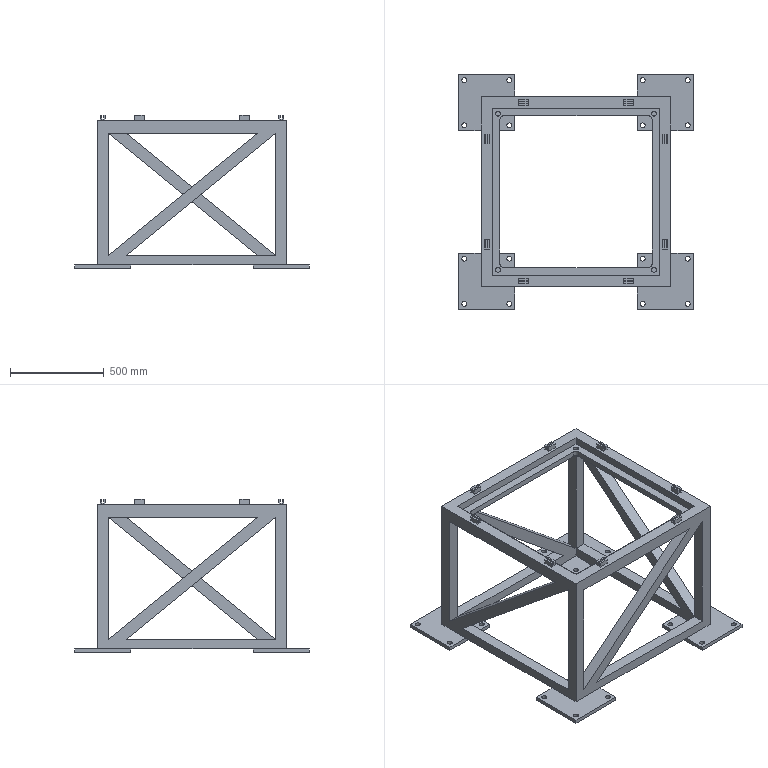Part | SolidWorks | features ICE 8, CirPattern 3, Extrusion 1, Fillet 1 | 1 solid | 187 faces | box 1250 x 1250 x 815 mm | volume 62783238 mm3 | plane 143 | cylinder 44 | commonest cylinder face diameters 26 x40 40 x4